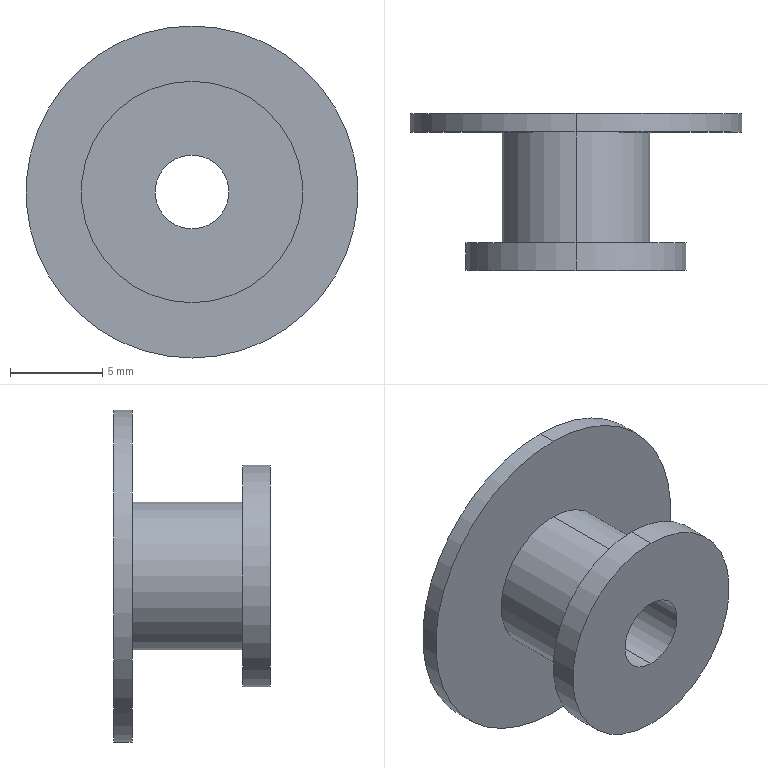Part | SolidWorks | features Revolution 1 | 1 solid | 12 faces | box 18 x 8.5 x 18 mm | volume 618.894 mm3 | cylinder 8 | plane 4 | commonest cylinder face diameters 4 x2 8 x2 12 x2 18 x2
STEP:
#1=CARTESIAN_POINT('',(0.,6.,-4.));
#2=VERTEX_POINT('',#1);
#3=CARTESIAN_POINT('',(0.,6.,4.));
#4=VERTEX_POINT('',#3);
#5=CARTESIAN_POINT('',(0.,6.,0.));
#6=DIRECTION('',(0.,-1.,0.));
#7=DIRECTION('',(0.,0.,-1.));
#8=AXIS2_PLACEMENT_3D('',#5,#6,#7);
#9=CIRCLE('',#8,4.);
#10=EDGE_CURVE('',#2,#4,#9,.T.);
#11=ORIENTED_EDGE('',*,*,#10,.T.);
#12=CARTESIAN_POINT('',(0.,0.,4.));
#13=VERTEX_POINT('',#12);
#14=CARTESIAN_POINT('',(0.,0.,4.));
#15=DIRECTION('',(0.,-1.,0.));
#16=VECTOR('',#15,1000.);
#17=LINE('',#14,#16);
#18=EDGE_CURVE('',#4,#13,#17,.T.);
#19=ORIENTED_EDGE('',*,*,#18,.T.);
#20=CARTESIAN_POINT('',(0.,0.,-4.));
#21=VERTEX_POINT('',#20);
#22=CARTESIAN_POINT('',(0.,0.,0.));
#23=DIRECTION('',(0.,-1.,0.));
#24=DIRECTION('',(0.,0.,-1.));
#25=AXIS2_PLACEMENT_3D('',#22,#23,#24);
#26=CIRCLE('',#25,4.);
#27=EDGE_CURVE('',#21,#13,#26,.T.);
#28=ORIENTED_EDGE('',*,*,#27,.F.);
#29=CARTESIAN_POINT('',(0.,0.,-4.));
#30=DIRECTION('',(0.,-1.,0.));
#31=VECTOR('',#30,1000.);
#32=LINE('',#29,#31);
#33=EDGE_CURVE('',#2,#21,#32,.T.);
#34=ORIENTED_EDGE('',*,*,#33,.F.);
#35=EDGE_LOOP('',(#11,#19,#28,#34));
#36=FACE_OUTER_BOUND('',#35,.T.);
#37=CARTESIAN_POINT('',(0.,0.,0.));
#38=DIRECTION('',(0.,-1.,0.));
#39=DIRECTION('',(0.,0.,-1.));
#40=AXIS2_PLACEMENT_3D('',#37,#38,#39);
#41=CYLINDRICAL_SURFACE('',#40,4.);
#42=ADVANCED_FACE('',(#36),#41,.T.);
#43=CARTESIAN_POINT('',(0.,0.,-6.));
#44=VERTEX_POINT('',#43);
#45=CARTESIAN_POINT('',(0.,0.,6.));
#46=VERTEX_POINT('',#45);
#47=CARTESIAN_POINT('',(0.,0.,0.));
#48=DIRECTION('',(0.,-1.,0.));
#49=DIRECTION('',(0.,0.,-1.));
#50=AXIS2_PLACEMENT_3D('',#47,#48,#49);
#51=CIRCLE('',#50,6.);
#52=EDGE_CURVE('',#44,#46,#51,.T.);
#53=ORIENTED_EDGE('',*,*,#52,.T.);
#54=CARTESIAN_POINT('',(0.,-1.5,6.));
#55=VERTEX_POINT('',#54);
#56=CARTESIAN_POINT('',(0.,0.,6.));
#57=DIRECTION('',(0.,-1.,0.));
#58=VECTOR('',#57,1000.);
#59=LINE('',#56,#58);
#60=EDGE_CURVE('',#46,#55,#59,.T.);
#61=ORIENTED_EDGE('',*,*,#60,.T.);
#62=CARTESIAN_POINT('',(0.,-1.5,-6.));
#63=VERTEX_POINT('',#62);
#64=CARTESIAN_POINT('',(0.,-1.5,0.));
#65=DIRECTION('',(0.,-1.,0.));
#66=DIRECTION('',(0.,0.,-1.));
#67=AXIS2_PLACEMENT_3D('',#64,#65,#66);
#68=CIRCLE('',#67,6.);
#69=EDGE_CURVE('',#63,#55,#68,.T.);
#70=ORIENTED_EDGE('',*,*,#69,.F.);
#71=CARTESIAN_POINT('',(0.,0.,-6.));
#72=DIRECTION('',(0.,-1.,0.));
#73=VECTOR('',#72,1000.);
#74=LINE('',#71,#73);
#75=EDGE_CURVE('',#44,#63,#74,.T.);
#76=ORIENTED_EDGE('',*,*,#75,.F.);
#77=EDGE_LOOP('',(#53,#61,#70,#76));
#78=FACE_OUTER_BOUND('',#77,.T.);
#79=CARTESIAN_POINT('',(0.,0.,0.));
#80=DIRECTION('',(0.,-1.,0.));
#81=DIRECTION('',(0.,0.,-1.));
#82=AXIS2_PLACEMENT_3D('',#79,#80,#81);
#83=CYLINDRICAL_SURFACE('',#82,6.);
#84=ADVANCED_FACE('',(#78),#83,.T.);
#85=CARTESIAN_POINT('',(0.,7.,2.));
#86=VERTEX_POINT('',#85);
#87=CARTESIAN_POINT('',(0.,7.,-2.));
#88=VERTEX_POINT('',#87);
#89=CARTESIAN_POINT('',(0.,7.,0.));
#90=DIRECTION('',(0.,-1.,0.));
#91=DIRECTION('',(0.,0.,-1.));
#92=AXIS2_PLACEMENT_3D('',#89,#90,#91);
#93=CIRCLE('',#92,2.);
#94=EDGE_CURVE('',#86,#88,#93,.T.);
#95=ORIENTED_EDGE('',*,*,#94,.F.);
#96=CARTESIAN_POINT('',(0.,-1.5,2.));
#97=VERTEX_POINT('',#96);
#98=CARTESIAN_POINT('',(0.,0.,2.));
#99=DIRECTION('',(0.,-1.,0.));
#100=VECTOR('',#99,1000.);
#101=LINE('',#98,#100);
#102=EDGE_CURVE('',#86,#97,#101,.T.);
#103=ORIENTED_EDGE('',*,*,#102,.T.);
#104=CARTESIAN_POINT('',(0.,-1.5,-2.));
#105=VERTEX_POINT('',#104);
#106=CARTESIAN_POINT('',(0.,-1.5,0.));
#107=DIRECTION('',(0.,-1.,0.));
#108=DIRECTION('',(0.,0.,-1.));
#109=AXIS2_PLACEMENT_3D('',#106,#107,#108);
#110=CIRCLE('',#109,2.);
#111=EDGE_CURVE('',#97,#105,#110,.T.);
#112=ORIENTED_EDGE('',*,*,#111,.T.);
#113=CARTESIAN_POINT('',(0.,0.,-2.));
#114=DIRECTION('',(0.,-1.,0.));
#115=VECTOR('',#114,1000.);
#116=LINE('',#113,#115);
#117=EDGE_CURVE('',#88,#105,#116,.T.);
#118=ORIENTED_EDGE('',*,*,#117,.F.);
#119=EDGE_LOOP('',(#95,#103,#112,#118));
#120=FACE_OUTER_BOUND('',#119,.T.);
#121=CARTESIAN_POINT('',(0.,0.,0.));
#122=DIRECTION('',(0.,-1.,0.));
#123=DIRECTION('',(0.,0.,-1.));
#124=AXIS2_PLACEMENT_3D('',#121,#122,#123);
#125=CYLINDRICAL_SURFACE('',#124,2.);
#126=ADVANCED_FACE('',(#120),#125,.F.);
#127=CARTESIAN_POINT('',(0.,7.,-9.));
#128=VERTEX_POINT('',#127);
#129=CARTESIAN_POINT('',(0.,7.,9.));
#130=VERTEX_POINT('',#129);
#131=CARTESIAN_POINT('',(0.,7.,0.));
#132=DIRECTION('',(0.,-1.,0.));
#133=DIRECTION('',(0.,0.,-1.));
#134=AXIS2_PLACEMENT_3D('',#131,#132,#133);
#135=CIRCLE('',#134,9.);
#136=EDGE_CURVE('',#128,#130,#135,.T.);
#137=ORIENTED_EDGE('',*,*,#136,.T.);
#138=CARTESIAN_POINT('',(0.,6.,9.));
#139=VERTEX_POINT('',#138);
#140=CARTESIAN_POINT('',(0.,0.,9.));
#141=DIRECTION('',(0.,-1.,0.));
#142=VECTOR('',#141,1000.);
#143=LINE('',#140,#142);
#144=EDGE_CURVE('',#130,#139,#143,.T.);
#145=ORIENTED_EDGE('',*,*,#144,.T.);
#146=CARTESIAN_POINT('',(0.,6.,-9.));
#147=VERTEX_POINT('',#146);
#148=CARTESIAN_POINT('',(0.,6.,0.));
#149=DIRECTION('',(0.,-1.,0.));
#150=DIRECTION('',(0.,0.,-1.));
#151=AXIS2_PLACEMENT_3D('',#148,#149,#150);
#152=CIRCLE('',#151,9.);
#153=EDGE_CURVE('',#147,#139,#152,.T.);
#154=ORIENTED_EDGE('',*,*,#153,.F.);
#155=CARTESIAN_POINT('',(0.,0.,-9.));
#156=DIRECTION('',(0.,-1.,0.));
#157=VECTOR('',#156,1000.);
#158=LINE('',#155,#157);
#159=EDGE_CURVE('',#128,#147,#158,.T.);
#160=ORIENTED_EDGE('',*,*,#159,.F.);
#161=EDGE_LOOP('',(#137,#145,#154,#160));
#162=FACE_OUTER_BOUND('',#161,.T.);
#163=CARTESIAN_POINT('',(0.,0.,0.));
#164=DIRECTION('',(0.,-1.,0.));
#165=DIRECTION('',(0.,0.,-1.));
#166=AXIS2_PLACEMENT_3D('',#163,#164,#165);
#167=CYLINDRICAL_SURFACE('',#166,9.);
#168=ADVANCED_FACE('',(#162),#167,.T.);
#169=ORIENTED_EDGE('',*,*,#153,.T.);
#170=CARTESIAN_POINT('',(0.,6.,0.));
#171=DIRECTION('',(0.,-1.,0.));
#172=DIRECTION('',(0.,0.,-1.));
#173=AXIS2_PLACEMENT_3D('',#170,#171,#172);
#174=CIRCLE('',#173,9.);
#175=EDGE_CURVE('',#139,#147,#174,.T.);
#176=ORIENTED_EDGE('',*,*,#175,.T.);
#177=EDGE_LOOP('',(#169,#176));
#178=FACE_OUTER_BOUND('',#177,.T.);
#179=ORIENTED_EDGE('',*,*,#10,.F.);
#180=CARTESIAN_POINT('',(0.,6.,0.));
#181=DIRECTION('',(0.,-1.,0.));
#182=DIRECTION('',(0.,0.,-1.));
#183=AXIS2_PLACEMENT_3D('',#180,#181,#182);
#184=CIRCLE('',#183,4.);
#185=EDGE_CURVE('',#4,#2,#184,.T.);
#186=ORIENTED_EDGE('',*,*,#185,.F.);
#187=EDGE_LOOP('',(#179,#186));
#188=FACE_BOUND('',#187,.T.);
#189=CARTESIAN_POINT('',(4.,6.,0.));
#190=DIRECTION('',(0.,-1.,0.));
#191=DIRECTION('',(0.,0.,-1.));
#192=AXIS2_PLACEMENT_3D('',#189,#190,#191);
#193=PLANE('',#192);
#194=ADVANCED_FACE('',(#178,#188),#193,.T.);
#195=ORIENTED_EDGE('',*,*,#144,.F.);
#196=CARTESIAN_POINT('',(0.,7.,0.));
#197=DIRECTION('',(0.,-1.,0.));
#198=DIRECTION('',(0.,0.,-1.));
#199=AXIS2_PLACEMENT_3D('',#196,#197,#198);
#200=CIRCLE('',#199,9.);
#201=EDGE_CURVE('',#130,#128,#200,.T.);
#202=ORIENTED_EDGE('',*,*,#201,.T.);
#203=ORIENTED_EDGE('',*,*,#159,.T.);
#204=ORIENTED_EDGE('',*,*,#175,.F.);
#205=EDGE_LOOP('',(#195,#202,#203,#204));
#206=FACE_OUTER_BOUND('',#205,.T.);
#207=CARTESIAN_POINT('',(0.,0.,0.));
#208=DIRECTION('',(0.,-1.,0.));
#209=DIRECTION('',(0.,0.,-1.));
#210=AXIS2_PLACEMENT_3D('',#207,#208,#209);
#211=CYLINDRICAL_SURFACE('',#210,9.);
#212=ADVANCED_FACE('',(#206),#211,.T.);
#213=CARTESIAN_POINT('',(0.,7.,0.));
#214=DIRECTION('',(0.,-1.,0.));
#215=DIRECTION('',(0.,0.,-1.));
#216=AXIS2_PLACEMENT_3D('',#213,#214,#215);
#217=CIRCLE('',#216,2.);
#218=EDGE_CURVE('',#88,#86,#217,.T.);
#219=ORIENTED_EDGE('',*,*,#218,.T.);
#220=ORIENTED_EDGE('',*,*,#94,.T.);
#221=EDGE_LOOP('',(#219,#220));
#222=FACE_BOUND('',#221,.T.);
#223=ORIENTED_EDGE('',*,*,#136,.F.);
#224=ORIENTED_EDGE('',*,*,#201,.F.);
#225=EDGE_LOOP('',(#223,#224));
#226=FACE_OUTER_BOUND('',#225,.T.);
#227=CARTESIAN_POINT('',(2.,7.,0.));
#228=DIRECTION('',(0.,1.,0.));
#229=DIRECTION('',(0.,0.,1.));
#230=AXIS2_PLACEMENT_3D('',#227,#228,#229);
#231=PLANE('',#230);
#232=ADVANCED_FACE('',(#222,#226),#231,.T.);
#233=ORIENTED_EDGE('',*,*,#102,.F.);
#234=ORIENTED_EDGE('',*,*,#218,.F.);
#235=ORIENTED_EDGE('',*,*,#117,.T.);
#236=CARTESIAN_POINT('',(0.,-1.5,0.));
#237=DIRECTION('',(0.,-1.,0.));
#238=DIRECTION('',(0.,0.,-1.));
#239=AXIS2_PLACEMENT_3D('',#236,#237,#238);
#240=CIRCLE('',#239,2.);
#241=EDGE_CURVE('',#105,#97,#240,.T.);
#242=ORIENTED_EDGE('',*,*,#241,.T.);
#243=EDGE_LOOP('',(#233,#234,#235,#242));
#244=FACE_OUTER_BOUND('',#243,.T.);
#245=CARTESIAN_POINT('',(0.,0.,0.));
#246=DIRECTION('',(0.,-1.,0.));
#247=DIRECTION('',(0.,0.,-1.));
#248=AXIS2_PLACEMENT_3D('',#245,#246,#247);
#249=CYLINDRICAL_SURFACE('',#248,2.);
#250=ADVANCED_FACE('',(#244),#249,.F.);
#251=ORIENTED_EDGE('',*,*,#69,.T.);
#252=CARTESIAN_POINT('',(0.,-1.5,0.));
#253=DIRECTION('',(0.,-1.,0.));
#254=DIRECTION('',(0.,0.,-1.));
#255=AXIS2_PLACEMENT_3D('',#252,#253,#254);
#256=CIRCLE('',#255,6.);
#257=EDGE_CURVE('',#55,#63,#256,.T.);
#258=ORIENTED_EDGE('',*,*,#257,.T.);
#259=EDGE_LOOP('',(#251,#258));
#260=FACE_OUTER_BOUND('',#259,.T.);
#261=ORIENTED_EDGE('',*,*,#241,.F.);
#262=ORIENTED_EDGE('',*,*,#111,.F.);
#263=EDGE_LOOP('',(#261,#262));
#264=FACE_BOUND('',#263,.T.);
#265=CARTESIAN_POINT('',(2.,-1.5,0.));
#266=DIRECTION('',(0.,-1.,0.));
#267=DIRECTION('',(0.,0.,-1.));
#268=AXIS2_PLACEMENT_3D('',#265,#266,#267);
#269=PLANE('',#268);
#270=ADVANCED_FACE('',(#260,#264),#269,.T.);
#271=ORIENTED_EDGE('',*,*,#60,.F.);
#272=CARTESIAN_POINT('',(0.,0.,0.));
#273=DIRECTION('',(0.,-1.,0.));
#274=DIRECTION('',(0.,0.,-1.));
#275=AXIS2_PLACEMENT_3D('',#272,#273,#274);
#276=CIRCLE('',#275,6.);
#277=EDGE_CURVE('',#46,#44,#276,.T.);
#278=ORIENTED_EDGE('',*,*,#277,.T.);
#279=ORIENTED_EDGE('',*,*,#75,.T.);
#280=ORIENTED_EDGE('',*,*,#257,.F.);
#281=EDGE_LOOP('',(#271,#278,#279,#280));
#282=FACE_OUTER_BOUND('',#281,.T.);
#283=CARTESIAN_POINT('',(0.,0.,0.));
#284=DIRECTION('',(0.,-1.,0.));
#285=DIRECTION('',(0.,0.,-1.));
#286=AXIS2_PLACEMENT_3D('',#283,#284,#285);
#287=CYLINDRICAL_SURFACE('',#286,6.);
#288=ADVANCED_FACE('',(#282),#287,.T.);
#289=ORIENTED_EDGE('',*,*,#27,.T.);
#290=CARTESIAN_POINT('',(0.,0.,0.));
#291=DIRECTION('',(0.,-1.,0.));
#292=DIRECTION('',(0.,0.,-1.));
#293=AXIS2_PLACEMENT_3D('',#290,#291,#292);
#294=CIRCLE('',#293,4.);
#295=EDGE_CURVE('',#13,#21,#294,.T.);
#296=ORIENTED_EDGE('',*,*,#295,.T.);
#297=EDGE_LOOP('',(#289,#296));
#298=FACE_BOUND('',#297,.T.);
#299=ORIENTED_EDGE('',*,*,#52,.F.);
#300=ORIENTED_EDGE('',*,*,#277,.F.);
#301=EDGE_LOOP('',(#299,#300));
#302=FACE_OUTER_BOUND('',#301,.T.);
#303=CARTESIAN_POINT('',(4.,0.,0.));
#304=DIRECTION('',(0.,1.,0.));
#305=DIRECTION('',(0.,0.,1.));
#306=AXIS2_PLACEMENT_3D('',#303,#304,#305);
#307=PLANE('',#306);
#308=ADVANCED_FACE('',(#298,#302),#307,.T.);
#309=ORIENTED_EDGE('',*,*,#18,.F.);
#310=ORIENTED_EDGE('',*,*,#185,.T.);
#311=ORIENTED_EDGE('',*,*,#33,.T.);
#312=ORIENTED_EDGE('',*,*,#295,.F.);
#313=EDGE_LOOP('',(#309,#310,#311,#312));
#314=FACE_OUTER_BOUND('',#313,.T.);
#315=CARTESIAN_POINT('',(0.,0.,0.));
#316=DIRECTION('',(0.,-1.,0.));
#317=DIRECTION('',(0.,0.,-1.));
#318=AXIS2_PLACEMENT_3D('',#315,#316,#317);
#319=CYLINDRICAL_SURFACE('',#318,4.);
#320=ADVANCED_FACE('',(#314),#319,.T.);
#321=CLOSED_SHELL('',(#42,#84,#126,#168,#194,#212,#232,#250,#270,#288,#308,#320));
#322=MANIFOLD_SOLID_BREP('',#321);
#323=CARTESIAN_POINT('',(0.,0.,0.));
#324=DIRECTION('',(0.,0.,1.));
#325=DIRECTION('',(1.,0.,0.));
#326=AXIS2_PLACEMENT_3D('',#323,#324,#325);
#327=(LENGTH_UNIT()NAMED_UNIT(*)SI_UNIT(.MILLI.,.METRE.));
#328=UNCERTAINTY_MEASURE_WITH_UNIT(LENGTH_MEASURE(0.00001),#327,'','');
#329=(NAMED_UNIT(*)PLANE_ANGLE_UNIT()SI_UNIT($,.RADIAN.));
#330=(NAMED_UNIT(*)SI_UNIT($,.STERADIAN.)SOLID_ANGLE_UNIT());
#331=(GEOMETRIC_REPRESENTATION_CONTEXT(3)GLOBAL_UNCERTAINTY_ASSIGNED_CONTEXT((#328))GLOBAL_UNIT_ASSIGNED_CONTEXT((#327,#329,#330))REPRESENTATION_CONTEXT('',''));
#332=ADVANCED_BREP_SHAPE_REPRESENTATION('',(#322,#326),#331);